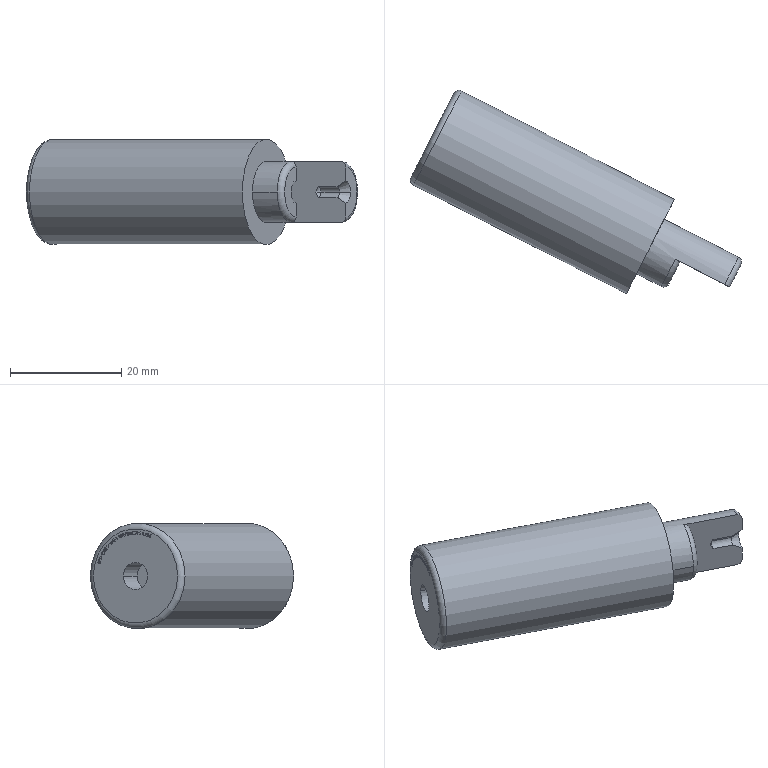Part | STEP file | 1_id470_x_t | 1 solid | 157 faces | box 59.58 x 36.56 x 19 mm | volume 13368 mm3 | plane 112 | other 25 | cylinder 9 | cone 8 | torus 3 | commonest cylinder face diameters 2 x4 4.9 x2 11 x2 19 x1